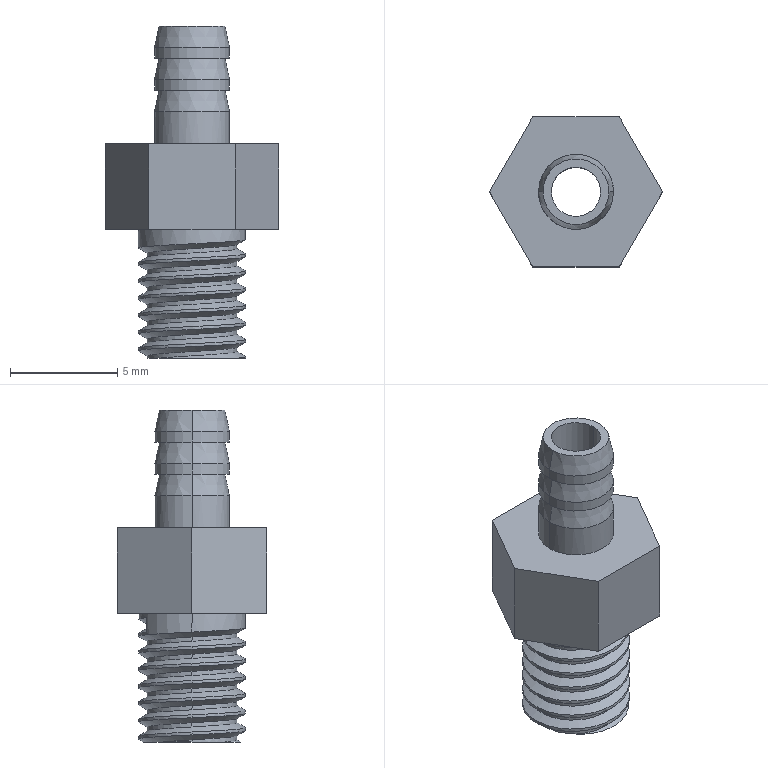Part | STEP file | 101000005928 | 1 solid | 59 faces | box 8.083 x 7 x 15.5 mm | volume 255.357 mm3 | cylinder 38 | plane 13 | cone 6 | spline 2 | commonest cylinder face diameters 4.2 x15 5 x15 3.5 x6 2.3 x2